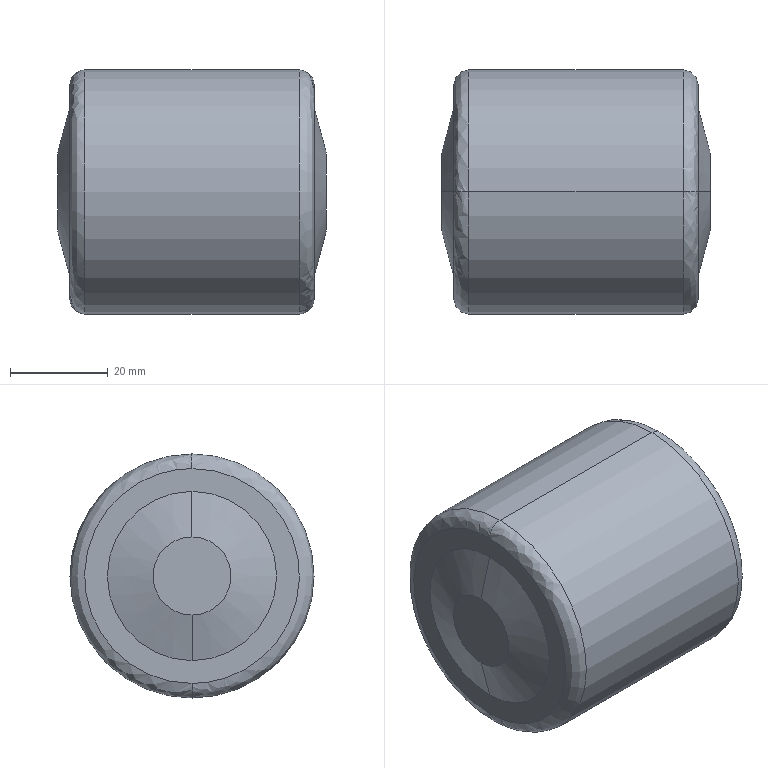Part | SolidWorks | features BaseBody 1 | 1 solid | 14 faces | box 55 x 50 x 50 mm | volume 100222 mm3 | spline 4 | cone 4 | plane 4 | cylinder 2 | commonest cylinder face diameters 50 x2
STEP:
#1=CARTESIAN_POINT('',(-22.,0.,25.));
#2=VERTEX_POINT('',#1);
#3=CARTESIAN_POINT('',(-22.,0.,-25.));
#4=VERTEX_POINT('',#3);
#5=CARTESIAN_POINT('',(-22.,0.,0.));
#6=DIRECTION('',(1.,0.,0.));
#7=DIRECTION('',(0.,0.,-1.));
#8=AXIS2_PLACEMENT_3D('',#5,#6,#7);
#9=CIRCLE('',#8,25.);
#10=EDGE_CURVE('',#2,#4,#9,.T.);
#11=ORIENTED_EDGE('',*,*,#10,.F.);
#12=CARTESIAN_POINT('',(-25.,0.,22.));
#13=VERTEX_POINT('',#12);
#14=CARTESIAN_POINT('',(-22.,0.,22.));
#15=DIRECTION('',(0.,-1.,0.));
#16=DIRECTION('',(0.,0.,1.));
#17=AXIS2_PLACEMENT_3D('',#14,#15,#16);
#18=CIRCLE('',#17,3.);
#19=EDGE_CURVE('',#2,#13,#18,.T.);
#20=ORIENTED_EDGE('',*,*,#19,.T.);
#21=CARTESIAN_POINT('',(-25.,0.,-22.));
#22=VERTEX_POINT('',#21);
#23=CARTESIAN_POINT('',(-25.,0.,22.));
#24=CARTESIAN_POINT('',(-25.,-44.,22.));
#25=CARTESIAN_POINT('',(-25.,-44.,-22.));
#26=CARTESIAN_POINT('',(-25.,0.,-22.));
#27=(BOUNDED_CURVE()B_SPLINE_CURVE(3,(#23,#24,#25,#26),.UNSPECIFIED.,.F.,.F.)B_SPLINE_CURVE_WITH_KNOTS((4,4),(0.5,1.),.UNSPECIFIED.)CURVE()GEOMETRIC_REPRESENTATION_ITEM()RATIONAL_B_SPLINE_CURVE((1.,0.3333,0.3333,1.))REPRESENTATION_ITEM(''));
#28=EDGE_CURVE('',#13,#22,#27,.T.);
#29=ORIENTED_EDGE('',*,*,#28,.T.);
#30=CARTESIAN_POINT('',(-22.,0.,-22.));
#31=DIRECTION('',(0.,1.,0.));
#32=DIRECTION('',(0.,0.,-1.));
#33=AXIS2_PLACEMENT_3D('',#30,#31,#32);
#34=CIRCLE('',#33,3.);
#35=EDGE_CURVE('',#4,#22,#34,.T.);
#36=ORIENTED_EDGE('',*,*,#35,.F.);
#37=EDGE_LOOP('',(#11,#20,#29,#36));
#38=FACE_OUTER_BOUND('',#37,.T.);
#39=CARTESIAN_POINT('',(-22.,0.,25.));
#40=CARTESIAN_POINT('',(-22.,-50.,25.));
#41=CARTESIAN_POINT('',(-22.,-50.,-25.));
#42=CARTESIAN_POINT('',(-22.,0.,-25.));
#43=CARTESIAN_POINT('',(-23.757,0.,25.));
#44=CARTESIAN_POINT('',(-23.757,-50.,25.));
#45=CARTESIAN_POINT('',(-23.757,-50.,-25.));
#46=CARTESIAN_POINT('',(-23.757,0.,-25.));
#47=CARTESIAN_POINT('',(-25.,0.,23.757));
#48=CARTESIAN_POINT('',(-25.,-47.515,23.757));
#49=CARTESIAN_POINT('',(-25.,-47.515,-23.757));
#50=CARTESIAN_POINT('',(-25.,0.,-23.757));
#51=CARTESIAN_POINT('',(-25.,0.,22.));
#52=CARTESIAN_POINT('',(-25.,-44.,22.));
#53=CARTESIAN_POINT('',(-25.,-44.,-22.));
#54=CARTESIAN_POINT('',(-25.,0.,-22.));
#55=(BOUNDED_SURFACE()B_SPLINE_SURFACE(3,3,((#39,#40,#41,#42),(#43,#44,#45,#46),(#47,#48,#49,#50),(#51,#52,#53,#54)),.UNSPECIFIED.,.F.,.F.,.F.)B_SPLINE_SURFACE_WITH_KNOTS((4,4),(4,4),(0.,1.),(0.,1.),.UNSPECIFIED.)GEOMETRIC_REPRESENTATION_ITEM()RATIONAL_B_SPLINE_SURFACE(((1.,0.3333,0.3333,1.),(0.8047,0.2682,0.2682,0.8047),(0.8047,0.2682,0.2682,0.8047),(1.,0.3333,0.3333,1.)))REPRESENTATION_ITEM('')SURFACE());
#56=ADVANCED_FACE('',(#38),#55,.T.);
#57=CARTESIAN_POINT('',(25.,0.,-22.));
#58=VERTEX_POINT('',#57);
#59=CARTESIAN_POINT('',(25.,0.,22.));
#60=VERTEX_POINT('',#59);
#61=CARTESIAN_POINT('',(25.,0.,-22.));
#62=CARTESIAN_POINT('',(25.,-44.,-22.));
#63=CARTESIAN_POINT('',(25.,-44.,22.));
#64=CARTESIAN_POINT('',(25.,0.,22.));
#65=(BOUNDED_CURVE()B_SPLINE_CURVE(3,(#61,#62,#63,#64),.UNSPECIFIED.,.F.,.F.)B_SPLINE_CURVE_WITH_KNOTS((4,4),(0.,0.5),.UNSPECIFIED.)CURVE()GEOMETRIC_REPRESENTATION_ITEM()RATIONAL_B_SPLINE_CURVE((1.,0.3333,0.3333,1.))REPRESENTATION_ITEM(''));
#66=EDGE_CURVE('',#58,#60,#65,.T.);
#67=ORIENTED_EDGE('',*,*,#66,.T.);
#68=CARTESIAN_POINT('',(22.,0.,25.));
#69=VERTEX_POINT('',#68);
#70=CARTESIAN_POINT('',(22.,0.,22.));
#71=DIRECTION('',(0.,-1.,0.));
#72=DIRECTION('',(0.,0.,1.));
#73=AXIS2_PLACEMENT_3D('',#70,#71,#72);
#74=CIRCLE('',#73,3.);
#75=EDGE_CURVE('',#60,#69,#74,.T.);
#76=ORIENTED_EDGE('',*,*,#75,.T.);
#77=CARTESIAN_POINT('',(22.,0.,-25.));
#78=VERTEX_POINT('',#77);
#79=CARTESIAN_POINT('',(22.,0.,0.));
#80=DIRECTION('',(-1.,0.,0.));
#81=DIRECTION('',(0.,0.,-1.));
#82=AXIS2_PLACEMENT_3D('',#79,#80,#81);
#83=CIRCLE('',#82,25.);
#84=EDGE_CURVE('',#78,#69,#83,.T.);
#85=ORIENTED_EDGE('',*,*,#84,.F.);
#86=CARTESIAN_POINT('',(22.,0.,-22.));
#87=DIRECTION('',(0.,1.,0.));
#88=DIRECTION('',(0.,0.,-1.));
#89=AXIS2_PLACEMENT_3D('',#86,#87,#88);
#90=CIRCLE('',#89,3.);
#91=EDGE_CURVE('',#58,#78,#90,.T.);
#92=ORIENTED_EDGE('',*,*,#91,.F.);
#93=EDGE_LOOP('',(#67,#76,#85,#92));
#94=FACE_OUTER_BOUND('',#93,.T.);
#95=CARTESIAN_POINT('',(25.,0.,22.));
#96=CARTESIAN_POINT('',(25.,-44.,22.));
#97=CARTESIAN_POINT('',(25.,-44.,-22.));
#98=CARTESIAN_POINT('',(25.,0.,-22.));
#99=CARTESIAN_POINT('',(25.,0.,23.757));
#100=CARTESIAN_POINT('',(25.,-47.515,23.757));
#101=CARTESIAN_POINT('',(25.,-47.515,-23.757));
#102=CARTESIAN_POINT('',(25.,0.,-23.757));
#103=CARTESIAN_POINT('',(23.757,0.,25.));
#104=CARTESIAN_POINT('',(23.757,-50.,25.));
#105=CARTESIAN_POINT('',(23.757,-50.,-25.));
#106=CARTESIAN_POINT('',(23.757,0.,-25.));
#107=CARTESIAN_POINT('',(22.,0.,25.));
#108=CARTESIAN_POINT('',(22.,-50.,25.));
#109=CARTESIAN_POINT('',(22.,-50.,-25.));
#110=CARTESIAN_POINT('',(22.,0.,-25.));
#111=(BOUNDED_SURFACE()B_SPLINE_SURFACE(3,3,((#95,#96,#97,#98),(#99,#100,#101,#102),(#103,#104,#105,#106),(#107,#108,#109,#110)),.UNSPECIFIED.,.F.,.F.,.T.)B_SPLINE_SURFACE_WITH_KNOTS((4,4),(4,4),(0.,1.),(0.,1.),.UNSPECIFIED.)GEOMETRIC_REPRESENTATION_ITEM()RATIONAL_B_SPLINE_SURFACE(((1.,0.3333,0.3333,1.),(0.8047,0.2682,0.2682,0.8047),(0.8047,0.2682,0.2682,0.8047),(1.,0.3333,0.3333,1.)))REPRESENTATION_ITEM('')SURFACE());
#112=ADVANCED_FACE('',(#94),#111,.T.);
#113=CARTESIAN_POINT('',(-22.,0.,0.));
#114=DIRECTION('',(1.,0.,0.));
#115=DIRECTION('',(0.,0.,-1.));
#116=AXIS2_PLACEMENT_3D('',#113,#114,#115);
#117=CIRCLE('',#116,25.);
#118=EDGE_CURVE('',#4,#2,#117,.T.);
#119=ORIENTED_EDGE('',*,*,#118,.T.);
#120=CARTESIAN_POINT('',(50.,0.,25.));
#121=DIRECTION('',(1.,0.,0.));
#122=VECTOR('',#121,1000.);
#123=LINE('',#120,#122);
#124=EDGE_CURVE('',#2,#69,#123,.T.);
#125=ORIENTED_EDGE('',*,*,#124,.T.);
#126=CARTESIAN_POINT('',(22.,0.,0.));
#127=DIRECTION('',(-1.,0.,0.));
#128=DIRECTION('',(0.,0.,-1.));
#129=AXIS2_PLACEMENT_3D('',#126,#127,#128);
#130=CIRCLE('',#129,25.);
#131=EDGE_CURVE('',#69,#78,#130,.T.);
#132=ORIENTED_EDGE('',*,*,#131,.T.);
#133=CARTESIAN_POINT('',(50.,0.,-25.));
#134=DIRECTION('',(1.,0.,0.));
#135=VECTOR('',#134,1000.);
#136=LINE('',#133,#135);
#137=EDGE_CURVE('',#4,#78,#136,.T.);
#138=ORIENTED_EDGE('',*,*,#137,.F.);
#139=EDGE_LOOP('',(#119,#125,#132,#138));
#140=FACE_OUTER_BOUND('',#139,.T.);
#141=CARTESIAN_POINT('',(50.,0.,0.));
#142=DIRECTION('',(1.,0.,0.));
#143=DIRECTION('',(0.,0.,-1.));
#144=AXIS2_PLACEMENT_3D('',#141,#142,#143);
#145=CYLINDRICAL_SURFACE('',#144,25.);
#146=ADVANCED_FACE('',(#140),#145,.T.);
#147=CARTESIAN_POINT('',(-27.5,0.,-8.));
#148=VERTEX_POINT('',#147);
#149=CARTESIAN_POINT('',(-27.5,0.,8.));
#150=VERTEX_POINT('',#149);
#151=CARTESIAN_POINT('',(-27.5,0.,0.));
#152=DIRECTION('',(1.,0.,0.));
#153=DIRECTION('',(0.,0.,-1.));
#154=AXIS2_PLACEMENT_3D('',#151,#152,#153);
#155=CIRCLE('',#154,8.);
#156=EDGE_CURVE('',#148,#150,#155,.T.);
#157=ORIENTED_EDGE('',*,*,#156,.T.);
#158=CARTESIAN_POINT('',(-25.,0.,17.33));
#159=VERTEX_POINT('',#158);
#160=CARTESIAN_POINT('',(-25.,0.,17.33));
#161=DIRECTION('',(0.2588,0.,0.9659));
#162=VECTOR('',#161,1000.);
#163=LINE('',#160,#162);
#164=EDGE_CURVE('',#150,#159,#163,.T.);
#165=ORIENTED_EDGE('',*,*,#164,.T.);
#166=CARTESIAN_POINT('',(-25.,0.,-17.33));
#167=VERTEX_POINT('',#166);
#168=CARTESIAN_POINT('',(-25.,0.,0.));
#169=DIRECTION('',(-1.,0.,0.));
#170=DIRECTION('',(0.,0.,-1.));
#171=AXIS2_PLACEMENT_3D('',#168,#169,#170);
#172=CIRCLE('',#171,17.33);
#173=EDGE_CURVE('',#159,#167,#172,.T.);
#174=ORIENTED_EDGE('',*,*,#173,.T.);
#175=CARTESIAN_POINT('',(-25.,0.,-17.33));
#176=DIRECTION('',(0.2588,0.,-0.9659));
#177=VECTOR('',#176,1000.);
#178=LINE('',#175,#177);
#179=EDGE_CURVE('',#148,#167,#178,.T.);
#180=ORIENTED_EDGE('',*,*,#179,.F.);
#181=EDGE_LOOP('',(#157,#165,#174,#180));
#182=FACE_OUTER_BOUND('',#181,.T.);
#183=CARTESIAN_POINT('',(-25.,0.,0.));
#184=DIRECTION('',(1.,0.,0.));
#185=DIRECTION('',(0.,0.,-1.));
#186=AXIS2_PLACEMENT_3D('',#183,#184,#185);
#187=CONICAL_SURFACE('',#186,17.33,1.309);
#188=ADVANCED_FACE('',(#182),#187,.T.);
#189=CARTESIAN_POINT('',(27.5,0.,8.));
#190=VERTEX_POINT('',#189);
#191=CARTESIAN_POINT('',(27.5,0.,-8.));
#192=VERTEX_POINT('',#191);
#193=CARTESIAN_POINT('',(27.5,0.,0.));
#194=DIRECTION('',(-1.,0.,0.));
#195=DIRECTION('',(0.,0.,1.));
#196=AXIS2_PLACEMENT_3D('',#193,#194,#195);
#197=CIRCLE('',#196,8.);
#198=EDGE_CURVE('',#190,#192,#197,.T.);
#199=ORIENTED_EDGE('',*,*,#198,.T.);
#200=CARTESIAN_POINT('',(25.,0.,-17.33));
#201=VERTEX_POINT('',#200);
#202=CARTESIAN_POINT('',(25.,0.,-17.33));
#203=DIRECTION('',(-0.2588,0.,-0.9659));
#204=VECTOR('',#203,1000.);
#205=LINE('',#202,#204);
#206=EDGE_CURVE('',#192,#201,#205,.T.);
#207=ORIENTED_EDGE('',*,*,#206,.T.);
#208=CARTESIAN_POINT('',(25.,0.,17.33));
#209=VERTEX_POINT('',#208);
#210=CARTESIAN_POINT('',(25.,0.,0.));
#211=DIRECTION('',(1.,0.,0.));
#212=DIRECTION('',(0.,0.,1.));
#213=AXIS2_PLACEMENT_3D('',#210,#211,#212);
#214=CIRCLE('',#213,17.33);
#215=EDGE_CURVE('',#201,#209,#214,.T.);
#216=ORIENTED_EDGE('',*,*,#215,.T.);
#217=CARTESIAN_POINT('',(25.,0.,17.33));
#218=DIRECTION('',(-0.2588,0.,0.9659));
#219=VECTOR('',#218,1000.);
#220=LINE('',#217,#219);
#221=EDGE_CURVE('',#190,#209,#220,.T.);
#222=ORIENTED_EDGE('',*,*,#221,.F.);
#223=EDGE_LOOP('',(#199,#207,#216,#222));
#224=FACE_OUTER_BOUND('',#223,.T.);
#225=CARTESIAN_POINT('',(25.,0.,0.));
#226=DIRECTION('',(-1.,0.,0.));
#227=DIRECTION('',(0.,0.,1.));
#228=AXIS2_PLACEMENT_3D('',#225,#226,#227);
#229=CONICAL_SURFACE('',#228,17.33,1.309);
#230=ADVANCED_FACE('',(#224),#229,.T.);
#231=ORIENTED_EDGE('',*,*,#124,.F.);
#232=ORIENTED_EDGE('',*,*,#10,.T.);
#233=ORIENTED_EDGE('',*,*,#137,.T.);
#234=ORIENTED_EDGE('',*,*,#84,.T.);
#235=EDGE_LOOP('',(#231,#232,#233,#234));
#236=FACE_OUTER_BOUND('',#235,.T.);
#237=CARTESIAN_POINT('',(50.,0.,0.));
#238=DIRECTION('',(1.,0.,0.));
#239=DIRECTION('',(0.,0.,-1.));
#240=AXIS2_PLACEMENT_3D('',#237,#238,#239);
#241=CYLINDRICAL_SURFACE('',#240,25.);
#242=ADVANCED_FACE('',(#236),#241,.T.);
#243=ORIENTED_EDGE('',*,*,#19,.F.);
#244=ORIENTED_EDGE('',*,*,#118,.F.);
#245=ORIENTED_EDGE('',*,*,#35,.T.);
#246=CARTESIAN_POINT('',(-25.,0.,-22.));
#247=CARTESIAN_POINT('',(-25.,44.,-22.));
#248=CARTESIAN_POINT('',(-25.,44.,22.));
#249=CARTESIAN_POINT('',(-25.,0.,22.));
#250=(BOUNDED_CURVE()B_SPLINE_CURVE(3,(#246,#247,#248,#249),.UNSPECIFIED.,.F.,.T.)B_SPLINE_CURVE_WITH_KNOTS((4,4),(0.,0.5),.UNSPECIFIED.)CURVE()GEOMETRIC_REPRESENTATION_ITEM()RATIONAL_B_SPLINE_CURVE((1.,0.3333,0.3333,1.))REPRESENTATION_ITEM(''));
#251=EDGE_CURVE('',#22,#13,#250,.T.);
#252=ORIENTED_EDGE('',*,*,#251,.T.);
#253=EDGE_LOOP('',(#243,#244,#245,#252));
#254=FACE_OUTER_BOUND('',#253,.T.);
#255=CARTESIAN_POINT('',(-22.,0.,-25.));
#256=CARTESIAN_POINT('',(-22.,50.,-25.));
#257=CARTESIAN_POINT('',(-22.,50.,25.));
#258=CARTESIAN_POINT('',(-22.,0.,25.));
#259=CARTESIAN_POINT('',(-23.757,0.,-25.));
#260=CARTESIAN_POINT('',(-23.757,50.,-25.));
#261=CARTESIAN_POINT('',(-23.757,50.,25.));
#262=CARTESIAN_POINT('',(-23.757,0.,25.));
#263=CARTESIAN_POINT('',(-25.,0.,-23.757));
#264=CARTESIAN_POINT('',(-25.,47.515,-23.757));
#265=CARTESIAN_POINT('',(-25.,47.515,23.757));
#266=CARTESIAN_POINT('',(-25.,0.,23.757));
#267=CARTESIAN_POINT('',(-25.,0.,-22.));
#268=CARTESIAN_POINT('',(-25.,44.,-22.));
#269=CARTESIAN_POINT('',(-25.,44.,22.));
#270=CARTESIAN_POINT('',(-25.,0.,22.));
#271=(BOUNDED_SURFACE()B_SPLINE_SURFACE(3,3,((#255,#256,#257,#258),(#259,#260,#261,#262),(#263,#264,#265,#266),(#267,#268,#269,#270)),.UNSPECIFIED.,.F.,.F.,.F.)B_SPLINE_SURFACE_WITH_KNOTS((4,4),(4,4),(0.,1.),(0.,1.),.UNSPECIFIED.)GEOMETRIC_REPRESENTATION_ITEM()RATIONAL_B_SPLINE_SURFACE(((1.,0.3333,0.3333,1.),(0.8047,0.2682,0.2682,0.8047),(0.8047,0.2682,0.2682,0.8047),(1.,0.3333,0.3333,1.)))REPRESENTATION_ITEM('')SURFACE());
#272=ADVANCED_FACE('',(#254),#271,.T.);
#273=ORIENTED_EDGE('',*,*,#75,.F.);
#274=CARTESIAN_POINT('',(25.,0.,22.));
#275=CARTESIAN_POINT('',(25.,44.,22.));
#276=CARTESIAN_POINT('',(25.,44.,-22.));
#277=CARTESIAN_POINT('',(25.,0.,-22.));
#278=(BOUNDED_CURVE()B_SPLINE_CURVE(3,(#274,#275,#276,#277),.UNSPECIFIED.,.F.,.F.)B_SPLINE_CURVE_WITH_KNOTS((4,4),(0.5,1.),.UNSPECIFIED.)CURVE()GEOMETRIC_REPRESENTATION_ITEM()RATIONAL_B_SPLINE_CURVE((1.,0.3333,0.3333,1.))REPRESENTATION_ITEM(''));
#279=EDGE_CURVE('',#60,#58,#278,.T.);
#280=ORIENTED_EDGE('',*,*,#279,.T.);
#281=ORIENTED_EDGE('',*,*,#91,.T.);
#282=ORIENTED_EDGE('',*,*,#131,.F.);
#283=EDGE_LOOP('',(#273,#280,#281,#282));
#284=FACE_OUTER_BOUND('',#283,.T.);
#285=CARTESIAN_POINT('',(25.,0.,-22.));
#286=CARTESIAN_POINT('',(25.,44.,-22.));
#287=CARTESIAN_POINT('',(25.,44.,22.));
#288=CARTESIAN_POINT('',(25.,0.,22.));
#289=CARTESIAN_POINT('',(25.,0.,-23.757));
#290=CARTESIAN_POINT('',(25.,47.515,-23.757));
#291=CARTESIAN_POINT('',(25.,47.515,23.757));
#292=CARTESIAN_POINT('',(25.,0.,23.757));
#293=CARTESIAN_POINT('',(23.757,0.,-25.));
#294=CARTESIAN_POINT('',(23.757,50.,-25.));
#295=CARTESIAN_POINT('',(23.757,50.,25.));
#296=CARTESIAN_POINT('',(23.757,0.,25.));
#297=CARTESIAN_POINT('',(22.,0.,-25.));
#298=CARTESIAN_POINT('',(22.,50.,-25.));
#299=CARTESIAN_POINT('',(22.,50.,25.));
#300=CARTESIAN_POINT('',(22.,0.,25.));
#301=(BOUNDED_SURFACE()B_SPLINE_SURFACE(3,3,((#285,#286,#287,#288),(#289,#290,#291,#292),(#293,#294,#295,#296),(#297,#298,#299,#300)),.UNSPECIFIED.,.F.,.F.,.F.)B_SPLINE_SURFACE_WITH_KNOTS((4,4),(4,4),(0.,1.),(0.,1.),.UNSPECIFIED.)GEOMETRIC_REPRESENTATION_ITEM()RATIONAL_B_SPLINE_SURFACE(((1.,0.3333,0.3333,1.),(0.8047,0.2682,0.2682,0.8047),(0.8047,0.2682,0.2682,0.8047),(1.,0.3333,0.3333,1.)))REPRESENTATION_ITEM('')SURFACE());
#302=ADVANCED_FACE('',(#284),#301,.T.);
#303=CARTESIAN_POINT('',(-25.,0.,0.));
#304=DIRECTION('',(-1.,0.,0.));
#305=DIRECTION('',(0.,0.,-1.));
#306=AXIS2_PLACEMENT_3D('',#303,#304,#305);
#307=CIRCLE('',#306,17.33);
#308=EDGE_CURVE('',#167,#159,#307,.T.);
#309=ORIENTED_EDGE('',*,*,#308,.F.);
#310=ORIENTED_EDGE('',*,*,#173,.F.);
#311=EDGE_LOOP('',(#309,#310));
#312=FACE_BOUND('',#311,.T.);
#313=ORIENTED_EDGE('',*,*,#251,.F.);
#314=ORIENTED_EDGE('',*,*,#28,.F.);
#315=EDGE_LOOP('',(#313,#314));
#316=FACE_OUTER_BOUND('',#315,.T.);
#317=CARTESIAN_POINT('',(-25.,17.33,0.));
#318=DIRECTION('',(1.,0.,0.));
#319=DIRECTION('',(0.,0.,-1.));
#320=AXIS2_PLACEMENT_3D('',#317,#318,#319);
#321=PLANE('',#320);
#322=ADVANCED_FACE('',(#312,#316),#321,.F.);
#323=ORIENTED_EDGE('',*,*,#66,.F.);
#324=ORIENTED_EDGE('',*,*,#279,.F.);
#325=EDGE_LOOP('',(#323,#324));
#326=FACE_OUTER_BOUND('',#325,.T.);
#327=CARTESIAN_POINT('',(25.,0.,0.));
#328=DIRECTION('',(1.,0.,0.));
#329=DIRECTION('',(0.,0.,1.));
#330=AXIS2_PLACEMENT_3D('',#327,#328,#329);
#331=CIRCLE('',#330,17.33);
#332=EDGE_CURVE('',#209,#201,#331,.T.);
#333=ORIENTED_EDGE('',*,*,#332,.F.);
#334=ORIENTED_EDGE('',*,*,#215,.F.);
#335=EDGE_LOOP('',(#333,#334));
#336=FACE_BOUND('',#335,.T.);
#337=CARTESIAN_POINT('',(25.,22.,0.));
#338=DIRECTION('',(-1.,0.,0.));
#339=DIRECTION('',(0.,0.,1.));
#340=AXIS2_PLACEMENT_3D('',#337,#338,#339);
#341=PLANE('',#340);
#342=ADVANCED_FACE('',(#326,#336),#341,.F.);
#343=ORIENTED_EDGE('',*,*,#164,.F.);
#344=CARTESIAN_POINT('',(-27.5,0.,0.));
#345=DIRECTION('',(1.,0.,0.));
#346=DIRECTION('',(0.,0.,-1.));
#347=AXIS2_PLACEMENT_3D('',#344,#345,#346);
#348=CIRCLE('',#347,8.);
#349=EDGE_CURVE('',#150,#148,#348,.T.);
#350=ORIENTED_EDGE('',*,*,#349,.T.);
#351=ORIENTED_EDGE('',*,*,#179,.T.);
#352=ORIENTED_EDGE('',*,*,#308,.T.);
#353=EDGE_LOOP('',(#343,#350,#351,#352));
#354=FACE_OUTER_BOUND('',#353,.T.);
#355=CARTESIAN_POINT('',(-25.,0.,0.));
#356=DIRECTION('',(1.,0.,0.));
#357=DIRECTION('',(0.,0.,-1.));
#358=AXIS2_PLACEMENT_3D('',#355,#356,#357);
#359=CONICAL_SURFACE('',#358,17.33,1.309);
#360=ADVANCED_FACE('',(#354),#359,.T.);
#361=ORIENTED_EDGE('',*,*,#206,.F.);
#362=CARTESIAN_POINT('',(27.5,0.,0.));
#363=DIRECTION('',(-1.,0.,0.));
#364=DIRECTION('',(0.,0.,1.));
#365=AXIS2_PLACEMENT_3D('',#362,#363,#364);
#366=CIRCLE('',#365,8.);
#367=EDGE_CURVE('',#192,#190,#366,.T.);
#368=ORIENTED_EDGE('',*,*,#367,.T.);
#369=ORIENTED_EDGE('',*,*,#221,.T.);
#370=ORIENTED_EDGE('',*,*,#332,.T.);
#371=EDGE_LOOP('',(#361,#368,#369,#370));
#372=FACE_OUTER_BOUND('',#371,.T.);
#373=CARTESIAN_POINT('',(25.,0.,0.));
#374=DIRECTION('',(-1.,0.,0.));
#375=DIRECTION('',(0.,0.,1.));
#376=AXIS2_PLACEMENT_3D('',#373,#374,#375);
#377=CONICAL_SURFACE('',#376,17.33,1.309);
#378=ADVANCED_FACE('',(#372),#377,.T.);
#379=ORIENTED_EDGE('',*,*,#156,.F.);
#380=ORIENTED_EDGE('',*,*,#349,.F.);
#381=EDGE_LOOP('',(#379,#380));
#382=FACE_OUTER_BOUND('',#381,.T.);
#383=CARTESIAN_POINT('',(-27.5,0.,0.));
#384=DIRECTION('',(1.,0.,0.));
#385=DIRECTION('',(0.,0.,-1.));
#386=AXIS2_PLACEMENT_3D('',#383,#384,#385);
#387=PLANE('',#386);
#388=ADVANCED_FACE('',(#382),#387,.F.);
#389=ORIENTED_EDGE('',*,*,#198,.F.);
#390=ORIENTED_EDGE('',*,*,#367,.F.);
#391=EDGE_LOOP('',(#389,#390));
#392=FACE_OUTER_BOUND('',#391,.T.);
#393=CARTESIAN_POINT('',(27.5,8.,0.));
#394=DIRECTION('',(-1.,0.,0.));
#395=DIRECTION('',(0.,0.,1.));
#396=AXIS2_PLACEMENT_3D('',#393,#394,#395);
#397=PLANE('',#396);
#398=ADVANCED_FACE('',(#392),#397,.F.);
#399=CLOSED_SHELL('',(#56,#112,#146,#188,#230,#242,#272,#302,#322,#342,#360,#378,#388,#398));
#400=MANIFOLD_SOLID_BREP('',#399);
#401=CARTESIAN_POINT('',(0.,0.,0.));
#402=DIRECTION('',(0.,0.,1.));
#403=DIRECTION('',(1.,0.,0.));
#404=AXIS2_PLACEMENT_3D('',#401,#402,#403);
#405=(LENGTH_UNIT()NAMED_UNIT(*)SI_UNIT(.MILLI.,.METRE.));
#406=UNCERTAINTY_MEASURE_WITH_UNIT(LENGTH_MEASURE(0.00001),#405,'','');
#407=(NAMED_UNIT(*)PLANE_ANGLE_UNIT()SI_UNIT($,.RADIAN.));
#408=(NAMED_UNIT(*)SI_UNIT($,.STERADIAN.)SOLID_ANGLE_UNIT());
#409=(GEOMETRIC_REPRESENTATION_CONTEXT(3)GLOBAL_UNCERTAINTY_ASSIGNED_CONTEXT((#406))GLOBAL_UNIT_ASSIGNED_CONTEXT((#405,#407,#408))REPRESENTATION_CONTEXT('',''));
#410=ADVANCED_BREP_SHAPE_REPRESENTATION('',(#400,#404),#409);